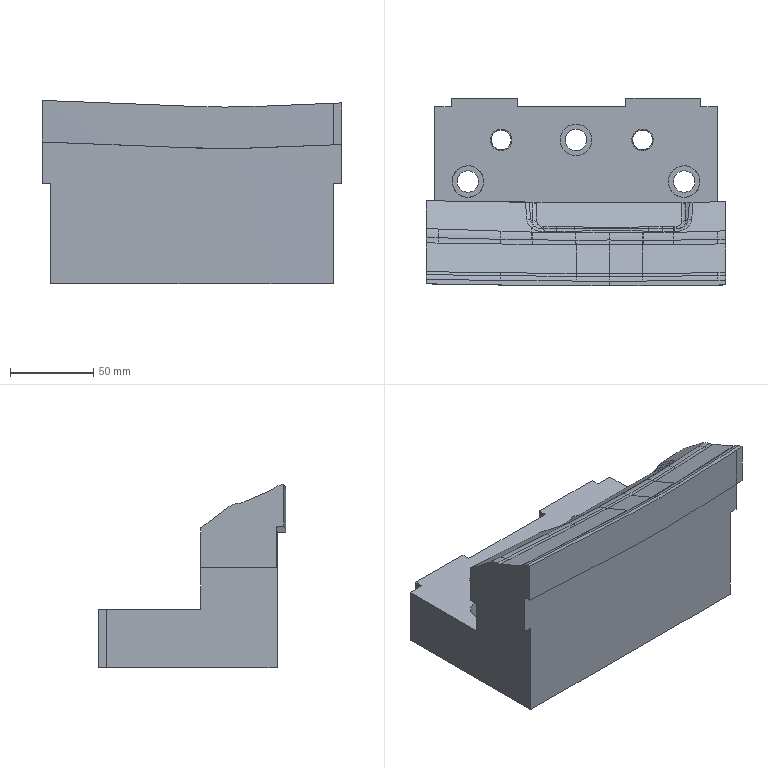Part | NX | features solid 2 | 1 solid | 120 faces | box 180 x 112.674 x 110.078 mm | volume 1093889 mm3 | spline 52 | cylinder 39 | plane 29 | commonest cylinder face diameters 20 x12 10 x8 13 x5 19 x3 12 x2 19.756 x2